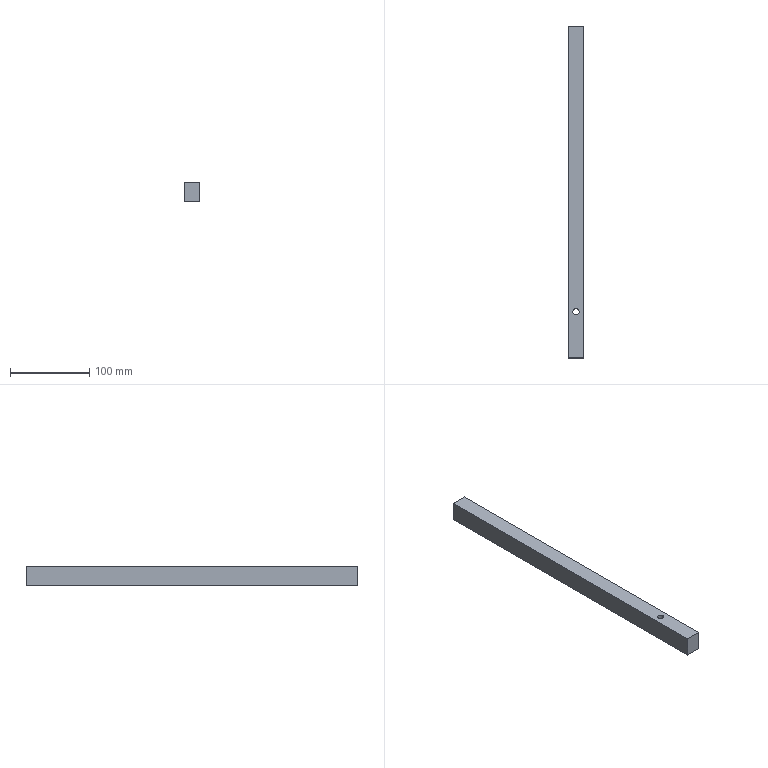Part | STEP file | lll_id3778_x_t | 1 solid | 7 faces | box 20 x 420 x 25 mm | volume 208743 mm3 | plane 6 | cylinder 1 | commonest cylinder face diameters 8 x1
STEP:
#1=CARTESIAN_POINT('',(4033.,-174.103,153.75));
#2=VERTEX_POINT('',#1);
#3=CARTESIAN_POINT('',(4033.,-594.103,153.75));
#4=VERTEX_POINT('',#3);
#5=CARTESIAN_POINT('',(4033.,-210.363,153.75));
#6=DIRECTION('',(0.,-1.,0.));
#7=VECTOR('',#6,1.);
#8=LINE('',#5,#7);
#9=EDGE_CURVE('',#2,#4,#8,.T.);
#10=ORIENTED_EDGE('',*,*,#9,.T.);
#11=CARTESIAN_POINT('',(4033.,-594.103,128.75));
#12=VERTEX_POINT('',#11);
#13=CARTESIAN_POINT('',(4033.,-594.103,158.75));
#14=DIRECTION('',(0.,0.,-1.));
#15=VECTOR('',#14,1.);
#16=LINE('',#13,#15);
#17=EDGE_CURVE('',#4,#12,#16,.T.);
#18=ORIENTED_EDGE('',*,*,#17,.T.);
#19=CARTESIAN_POINT('',(4033.,-174.103,128.75));
#20=VERTEX_POINT('',#19);
#21=CARTESIAN_POINT('',(4033.,-271.677,128.75));
#22=DIRECTION('',(0.,-1.,0.));
#23=VECTOR('',#22,1.);
#24=LINE('',#21,#23);
#25=EDGE_CURVE('',#20,#12,#24,.T.);
#26=ORIENTED_EDGE('',*,*,#25,.F.);
#27=CARTESIAN_POINT('',(4033.,-174.103,158.75));
#28=DIRECTION('',(0.,0.,1.));
#29=VECTOR('',#28,1.);
#30=LINE('',#27,#29);
#31=EDGE_CURVE('',#20,#2,#30,.T.);
#32=ORIENTED_EDGE('',*,*,#31,.T.);
#33=EDGE_LOOP('',(#10,#18,#26,#32));
#34=FACE_OUTER_BOUND('',#33,.T.);
#35=CARTESIAN_POINT('',(4033.,-210.363,158.75));
#36=DIRECTION('',(1.,0.,0.));
#37=DIRECTION('',(0.,-1.,0.));
#38=AXIS2_PLACEMENT_3D('',#35,#36,#37);
#39=PLANE('',#38);
#40=ADVANCED_FACE('',(#34),#39,.T.);
#41=CARTESIAN_POINT('',(4027.,-535.677,153.75));
#42=VERTEX_POINT('',#41);
#43=CARTESIAN_POINT('',(4023.,-535.677,153.75));
#44=DIRECTION('',(0.,0.,1.));
#45=DIRECTION('',(1.,0.,0.));
#46=AXIS2_PLACEMENT_3D('',#43,#44,#45);
#47=CIRCLE('',#46,4.);
#48=EDGE_CURVE('',#42,#42,#47,.T.);
#49=ORIENTED_EDGE('',*,*,#48,.F.);
#50=EDGE_LOOP('',(#49));
#51=FACE_BOUND('',#50,.T.);
#52=CARTESIAN_POINT('',(4013.,-594.103,153.75));
#53=VERTEX_POINT('',#52);
#54=CARTESIAN_POINT('',(4013.,-174.103,153.75));
#55=VERTEX_POINT('',#54);
#56=CARTESIAN_POINT('',(4013.,-210.103,153.75));
#57=DIRECTION('',(0.,1.,0.));
#58=VECTOR('',#57,1.);
#59=LINE('',#56,#58);
#60=EDGE_CURVE('',#53,#55,#59,.T.);
#61=ORIENTED_EDGE('',*,*,#60,.F.);
#62=CARTESIAN_POINT('',(4015.5,-594.103,153.75));
#63=DIRECTION('',(1.,0.,0.));
#64=VECTOR('',#63,1.);
#65=LINE('',#62,#64);
#66=EDGE_CURVE('',#53,#4,#65,.T.);
#67=ORIENTED_EDGE('',*,*,#66,.T.);
#68=ORIENTED_EDGE('',*,*,#9,.F.);
#69=CARTESIAN_POINT('',(4015.5,-174.103,153.75));
#70=DIRECTION('',(-1.,0.,0.));
#71=VECTOR('',#70,1.);
#72=LINE('',#69,#71);
#73=EDGE_CURVE('',#2,#55,#72,.T.);
#74=ORIENTED_EDGE('',*,*,#73,.T.);
#75=EDGE_LOOP('',(#61,#67,#68,#74));
#76=FACE_BOUND('',#75,.T.);
#77=CARTESIAN_POINT('',(4015.5,-377.103,153.75));
#78=DIRECTION('',(0.,0.,1.));
#79=DIRECTION('',(-1.,0.,0.));
#80=AXIS2_PLACEMENT_3D('',#77,#78,#79);
#81=PLANE('',#80);
#82=ADVANCED_FACE('',(#51,#76),#81,.T.);
#83=CARTESIAN_POINT('',(4027.,-535.677,128.75));
#84=VERTEX_POINT('',#83);
#85=CARTESIAN_POINT('',(4023.,-535.677,128.75));
#86=DIRECTION('',(0.,0.,1.));
#87=DIRECTION('',(1.,0.,0.));
#88=AXIS2_PLACEMENT_3D('',#85,#86,#87);
#89=CIRCLE('',#88,4.);
#90=EDGE_CURVE('',#84,#84,#89,.T.);
#91=ORIENTED_EDGE('',*,*,#90,.T.);
#92=EDGE_LOOP('',(#91));
#93=FACE_BOUND('',#92,.T.);
#94=CARTESIAN_POINT('',(4013.,-594.103,128.75));
#95=VERTEX_POINT('',#94);
#96=CARTESIAN_POINT('',(3157.,-594.103,128.75));
#97=DIRECTION('',(-1.,0.,0.));
#98=VECTOR('',#97,1.);
#99=LINE('',#96,#98);
#100=EDGE_CURVE('',#12,#95,#99,.T.);
#101=ORIENTED_EDGE('',*,*,#100,.T.);
#102=CARTESIAN_POINT('',(4013.,-174.103,128.75));
#103=VERTEX_POINT('',#102);
#104=CARTESIAN_POINT('',(4013.,-210.103,128.75));
#105=DIRECTION('',(0.,-1.,0.));
#106=VECTOR('',#105,1.);
#107=LINE('',#104,#106);
#108=EDGE_CURVE('',#103,#95,#107,.T.);
#109=ORIENTED_EDGE('',*,*,#108,.F.);
#110=CARTESIAN_POINT('',(3157.,-174.103,128.75));
#111=DIRECTION('',(1.,0.,0.));
#112=VECTOR('',#111,1.);
#113=LINE('',#110,#112);
#114=EDGE_CURVE('',#103,#20,#113,.T.);
#115=ORIENTED_EDGE('',*,*,#114,.T.);
#116=ORIENTED_EDGE('',*,*,#25,.T.);
#117=EDGE_LOOP('',(#101,#109,#115,#116));
#118=FACE_BOUND('',#117,.T.);
#119=CARTESIAN_POINT('',(3157.,-271.677,128.75));
#120=DIRECTION('',(0.,0.,1.));
#121=DIRECTION('',(-1.,0.,0.));
#122=AXIS2_PLACEMENT_3D('',#119,#120,#121);
#123=PLANE('',#122);
#124=ADVANCED_FACE('',(#93,#118),#123,.F.);
#125=ORIENTED_EDGE('',*,*,#108,.T.);
#126=CARTESIAN_POINT('',(4013.,-594.103,158.75));
#127=DIRECTION('',(0.,0.,1.));
#128=VECTOR('',#127,1.);
#129=LINE('',#126,#128);
#130=EDGE_CURVE('',#95,#53,#129,.T.);
#131=ORIENTED_EDGE('',*,*,#130,.T.);
#132=ORIENTED_EDGE('',*,*,#60,.T.);
#133=CARTESIAN_POINT('',(4013.,-174.103,158.75));
#134=DIRECTION('',(0.,0.,-1.));
#135=VECTOR('',#134,1.);
#136=LINE('',#133,#135);
#137=EDGE_CURVE('',#55,#103,#136,.T.);
#138=ORIENTED_EDGE('',*,*,#137,.T.);
#139=EDGE_LOOP('',(#125,#131,#132,#138));
#140=FACE_OUTER_BOUND('',#139,.T.);
#141=CARTESIAN_POINT('',(4013.,-210.103,158.75));
#142=DIRECTION('',(-1.,0.,0.));
#143=DIRECTION('',(0.,0.,1.));
#144=AXIS2_PLACEMENT_3D('',#141,#142,#143);
#145=PLANE('',#144);
#146=ADVANCED_FACE('',(#140),#145,.T.);
#147=ORIENTED_EDGE('',*,*,#31,.F.);
#148=ORIENTED_EDGE('',*,*,#114,.F.);
#149=ORIENTED_EDGE('',*,*,#137,.F.);
#150=ORIENTED_EDGE('',*,*,#73,.F.);
#151=EDGE_LOOP('',(#147,#148,#149,#150));
#152=FACE_OUTER_BOUND('',#151,.T.);
#153=CARTESIAN_POINT('',(4026.,-174.103,147.25));
#154=DIRECTION('',(0.,1.,0.));
#155=DIRECTION('',(0.,0.,1.));
#156=AXIS2_PLACEMENT_3D('',#153,#154,#155);
#157=PLANE('',#156);
#158=ADVANCED_FACE('',(#152),#157,.T.);
#159=ORIENTED_EDGE('',*,*,#66,.F.);
#160=ORIENTED_EDGE('',*,*,#130,.F.);
#161=ORIENTED_EDGE('',*,*,#100,.F.);
#162=ORIENTED_EDGE('',*,*,#17,.F.);
#163=EDGE_LOOP('',(#159,#160,#161,#162));
#164=FACE_OUTER_BOUND('',#163,.T.);
#165=CARTESIAN_POINT('',(4016.5,-594.103,141.25));
#166=DIRECTION('',(0.,-1.,0.));
#167=DIRECTION('',(0.,0.,-1.));
#168=AXIS2_PLACEMENT_3D('',#165,#166,#167);
#169=PLANE('',#168);
#170=ADVANCED_FACE('',(#164),#169,.T.);
#171=ORIENTED_EDGE('',*,*,#48,.T.);
#172=EDGE_LOOP('',(#171));
#173=FACE_BOUND('',#172,.T.);
#174=ORIENTED_EDGE('',*,*,#90,.F.);
#175=EDGE_LOOP('',(#174));
#176=FACE_BOUND('',#175,.T.);
#177=CARTESIAN_POINT('',(4023.,-535.677,170.));
#178=DIRECTION('',(0.,0.,-1.));
#179=DIRECTION('',(1.,0.,0.));
#180=AXIS2_PLACEMENT_3D('',#177,#178,#179);
#181=CYLINDRICAL_SURFACE('',#180,4.);
#182=ADVANCED_FACE('',(#173,#176),#181,.F.);
#183=CLOSED_SHELL('',(#40,#82,#124,#146,#158,#170,#182));
#184=MANIFOLD_SOLID_BREP('',#183);
#185=(LENGTH_UNIT()NAMED_UNIT(*)SI_UNIT(.MILLI.,.METRE.));
#186=UNCERTAINTY_MEASURE_WITH_UNIT(LENGTH_MEASURE(0.00002),#185,'','');
#187=(NAMED_UNIT(*)PLANE_ANGLE_UNIT()SI_UNIT($,.RADIAN.));
#188=PLANE_ANGLE_MEASURE_WITH_UNIT(PLANE_ANGLE_MEASURE(0.01745),#187);
#189=DIMENSIONAL_EXPONENTS(0.,0.,0.,0.,0.,0.,0.);
#190=(CONVERSION_BASED_UNIT('DEGREE',#188)NAMED_UNIT(#189)PLANE_ANGLE_UNIT());
#191=(NAMED_UNIT(*)SI_UNIT($,.STERADIAN.)SOLID_ANGLE_UNIT());
#192=(GEOMETRIC_REPRESENTATION_CONTEXT(3)GLOBAL_UNCERTAINTY_ASSIGNED_CONTEXT((#186))GLOBAL_UNIT_ASSIGNED_CONTEXT((#185,#190,#191))REPRESENTATION_CONTEXT('',''));
#193=ADVANCED_BREP_SHAPE_REPRESENTATION('',(#184),#192);